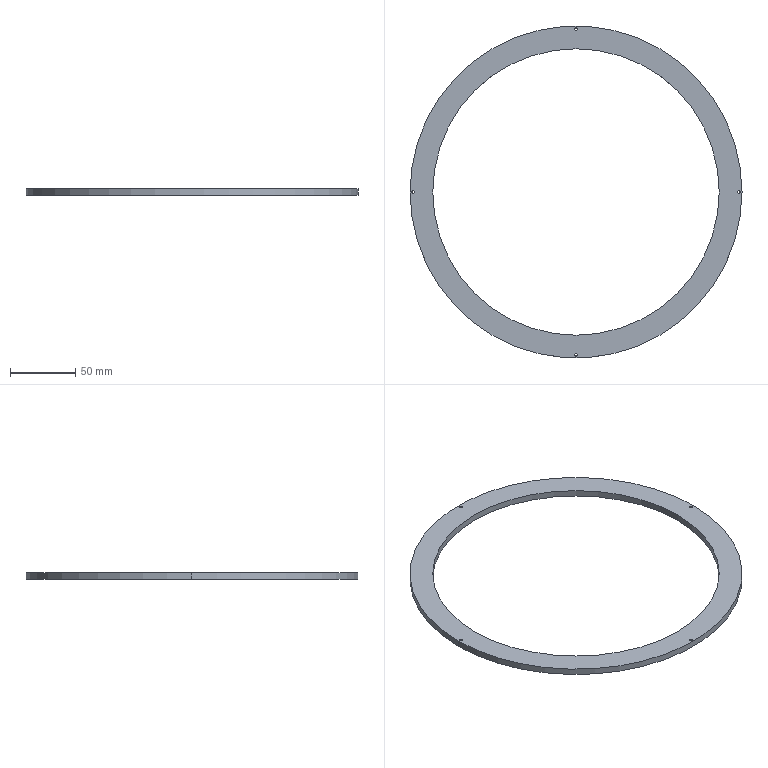Part | SolidWorks | features CirPattern 1, Extrusion 1, ICE 1 | 1 solid | 14 faces | box 255 x 255 x 5 mm | volume 65223 mm3 | cylinder 12 | plane 2 | commonest cylinder face diameters 2 x8 220 x2 255 x2
STEP:
#1=CARTESIAN_POINT('',(-126.,0.,0.));
#2=VERTEX_POINT('',#1);
#3=CARTESIAN_POINT('',(-124.,0.,0.));
#4=VERTEX_POINT('',#3);
#5=CARTESIAN_POINT('',(-125.,0.,0.));
#6=DIRECTION('',(0.,0.,1.));
#7=DIRECTION('',(0.,1.,0.));
#8=AXIS2_PLACEMENT_3D('',#5,#6,#7);
#9=CIRCLE('',#8,1.);
#10=EDGE_CURVE('',#2,#4,#9,.T.);
#11=ORIENTED_EDGE('',*,*,#10,.F.);
#12=CARTESIAN_POINT('',(-126.,0.,5.));
#13=VERTEX_POINT('',#12);
#14=CARTESIAN_POINT('',(-126.,0.,0.));
#15=DIRECTION('',(0.,0.,1.));
#16=VECTOR('',#15,1000.);
#17=LINE('',#14,#16);
#18=EDGE_CURVE('',#2,#13,#17,.T.);
#19=ORIENTED_EDGE('',*,*,#18,.T.);
#20=CARTESIAN_POINT('',(-124.,0.,5.));
#21=VERTEX_POINT('',#20);
#22=CARTESIAN_POINT('',(-125.,0.,5.));
#23=DIRECTION('',(0.,0.,1.));
#24=DIRECTION('',(0.,1.,0.));
#25=AXIS2_PLACEMENT_3D('',#22,#23,#24);
#26=CIRCLE('',#25,1.);
#27=EDGE_CURVE('',#13,#21,#26,.T.);
#28=ORIENTED_EDGE('',*,*,#27,.T.);
#29=CARTESIAN_POINT('',(-124.,0.,0.));
#30=DIRECTION('',(0.,0.,1.));
#31=VECTOR('',#30,1000.);
#32=LINE('',#29,#31);
#33=EDGE_CURVE('',#4,#21,#32,.T.);
#34=ORIENTED_EDGE('',*,*,#33,.F.);
#35=EDGE_LOOP('',(#11,#19,#28,#34));
#36=FACE_OUTER_BOUND('',#35,.T.);
#37=CARTESIAN_POINT('',(-125.,0.,0.));
#38=DIRECTION('',(0.,0.,1.));
#39=DIRECTION('',(1.,0.,0.));
#40=AXIS2_PLACEMENT_3D('',#37,#38,#39);
#41=CYLINDRICAL_SURFACE('',#40,1.);
#42=ADVANCED_FACE('',(#36),#41,.F.);
#43=CARTESIAN_POINT('',(-1.,-125.,0.));
#44=VERTEX_POINT('',#43);
#45=CARTESIAN_POINT('',(1.,-125.,0.));
#46=VERTEX_POINT('',#45);
#47=CARTESIAN_POINT('',(0.,-125.,0.));
#48=DIRECTION('',(0.,0.,1.));
#49=DIRECTION('',(-1.,0.,0.));
#50=AXIS2_PLACEMENT_3D('',#47,#48,#49);
#51=CIRCLE('',#50,1.);
#52=EDGE_CURVE('',#44,#46,#51,.T.);
#53=ORIENTED_EDGE('',*,*,#52,.F.);
#54=CARTESIAN_POINT('',(-1.,-125.,5.));
#55=VERTEX_POINT('',#54);
#56=CARTESIAN_POINT('',(-1.,-125.,0.));
#57=DIRECTION('',(0.,0.,1.));
#58=VECTOR('',#57,1000.);
#59=LINE('',#56,#58);
#60=EDGE_CURVE('',#44,#55,#59,.T.);
#61=ORIENTED_EDGE('',*,*,#60,.T.);
#62=CARTESIAN_POINT('',(1.,-125.,5.));
#63=VERTEX_POINT('',#62);
#64=CARTESIAN_POINT('',(0.,-125.,5.));
#65=DIRECTION('',(0.,0.,1.));
#66=DIRECTION('',(-1.,0.,0.));
#67=AXIS2_PLACEMENT_3D('',#64,#65,#66);
#68=CIRCLE('',#67,1.);
#69=EDGE_CURVE('',#55,#63,#68,.T.);
#70=ORIENTED_EDGE('',*,*,#69,.T.);
#71=CARTESIAN_POINT('',(1.,-125.,0.));
#72=DIRECTION('',(0.,0.,1.));
#73=VECTOR('',#72,1000.);
#74=LINE('',#71,#73);
#75=EDGE_CURVE('',#46,#63,#74,.T.);
#76=ORIENTED_EDGE('',*,*,#75,.F.);
#77=EDGE_LOOP('',(#53,#61,#70,#76));
#78=FACE_OUTER_BOUND('',#77,.T.);
#79=CARTESIAN_POINT('',(0.,-125.,0.));
#80=DIRECTION('',(0.,0.,1.));
#81=DIRECTION('',(1.,0.,0.));
#82=AXIS2_PLACEMENT_3D('',#79,#80,#81);
#83=CYLINDRICAL_SURFACE('',#82,1.);
#84=ADVANCED_FACE('',(#78),#83,.F.);
#85=CARTESIAN_POINT('',(124.,0.,0.));
#86=VERTEX_POINT('',#85);
#87=CARTESIAN_POINT('',(126.,0.,0.));
#88=VERTEX_POINT('',#87);
#89=CARTESIAN_POINT('',(125.,0.,0.));
#90=DIRECTION('',(0.,0.,1.));
#91=DIRECTION('',(0.,-1.,0.));
#92=AXIS2_PLACEMENT_3D('',#89,#90,#91);
#93=CIRCLE('',#92,1.);
#94=EDGE_CURVE('',#86,#88,#93,.T.);
#95=ORIENTED_EDGE('',*,*,#94,.F.);
#96=CARTESIAN_POINT('',(124.,0.,5.));
#97=VERTEX_POINT('',#96);
#98=CARTESIAN_POINT('',(124.,0.,0.));
#99=DIRECTION('',(0.,0.,1.));
#100=VECTOR('',#99,1000.);
#101=LINE('',#98,#100);
#102=EDGE_CURVE('',#86,#97,#101,.T.);
#103=ORIENTED_EDGE('',*,*,#102,.T.);
#104=CARTESIAN_POINT('',(126.,0.,5.));
#105=VERTEX_POINT('',#104);
#106=CARTESIAN_POINT('',(125.,0.,5.));
#107=DIRECTION('',(0.,0.,1.));
#108=DIRECTION('',(0.,-1.,0.));
#109=AXIS2_PLACEMENT_3D('',#106,#107,#108);
#110=CIRCLE('',#109,1.);
#111=EDGE_CURVE('',#97,#105,#110,.T.);
#112=ORIENTED_EDGE('',*,*,#111,.T.);
#113=CARTESIAN_POINT('',(126.,0.,0.));
#114=DIRECTION('',(0.,0.,1.));
#115=VECTOR('',#114,1000.);
#116=LINE('',#113,#115);
#117=EDGE_CURVE('',#88,#105,#116,.T.);
#118=ORIENTED_EDGE('',*,*,#117,.F.);
#119=EDGE_LOOP('',(#95,#103,#112,#118));
#120=FACE_OUTER_BOUND('',#119,.T.);
#121=CARTESIAN_POINT('',(125.,0.,0.));
#122=DIRECTION('',(0.,0.,1.));
#123=DIRECTION('',(1.,0.,0.));
#124=AXIS2_PLACEMENT_3D('',#121,#122,#123);
#125=CYLINDRICAL_SURFACE('',#124,1.);
#126=ADVANCED_FACE('',(#120),#125,.F.);
#127=CARTESIAN_POINT('',(-1.,125.,0.));
#128=VERTEX_POINT('',#127);
#129=CARTESIAN_POINT('',(1.,125.,0.));
#130=VERTEX_POINT('',#129);
#131=CARTESIAN_POINT('',(0.,125.,0.));
#132=DIRECTION('',(0.,0.,1.));
#133=DIRECTION('',(1.,0.,0.));
#134=AXIS2_PLACEMENT_3D('',#131,#132,#133);
#135=CIRCLE('',#134,1.);
#136=EDGE_CURVE('',#128,#130,#135,.T.);
#137=ORIENTED_EDGE('',*,*,#136,.F.);
#138=CARTESIAN_POINT('',(-1.,125.,5.));
#139=VERTEX_POINT('',#138);
#140=CARTESIAN_POINT('',(-1.,125.,0.));
#141=DIRECTION('',(0.,0.,1.));
#142=VECTOR('',#141,1000.);
#143=LINE('',#140,#142);
#144=EDGE_CURVE('',#128,#139,#143,.T.);
#145=ORIENTED_EDGE('',*,*,#144,.T.);
#146=CARTESIAN_POINT('',(1.,125.,5.));
#147=VERTEX_POINT('',#146);
#148=CARTESIAN_POINT('',(0.,125.,5.));
#149=DIRECTION('',(0.,0.,1.));
#150=DIRECTION('',(1.,0.,0.));
#151=AXIS2_PLACEMENT_3D('',#148,#149,#150);
#152=CIRCLE('',#151,1.);
#153=EDGE_CURVE('',#139,#147,#152,.T.);
#154=ORIENTED_EDGE('',*,*,#153,.T.);
#155=CARTESIAN_POINT('',(1.,125.,0.));
#156=DIRECTION('',(0.,0.,1.));
#157=VECTOR('',#156,1000.);
#158=LINE('',#155,#157);
#159=EDGE_CURVE('',#130,#147,#158,.T.);
#160=ORIENTED_EDGE('',*,*,#159,.F.);
#161=EDGE_LOOP('',(#137,#145,#154,#160));
#162=FACE_OUTER_BOUND('',#161,.T.);
#163=CARTESIAN_POINT('',(0.,125.,0.));
#164=DIRECTION('',(0.,0.,1.));
#165=DIRECTION('',(1.,0.,0.));
#166=AXIS2_PLACEMENT_3D('',#163,#164,#165);
#167=CYLINDRICAL_SURFACE('',#166,1.);
#168=ADVANCED_FACE('',(#162),#167,.F.);
#169=CARTESIAN_POINT('',(-110.,0.,5.));
#170=VERTEX_POINT('',#169);
#171=CARTESIAN_POINT('',(110.,0.,5.));
#172=VERTEX_POINT('',#171);
#173=CARTESIAN_POINT('',(0.,0.,5.));
#174=DIRECTION('',(0.,0.,1.));
#175=DIRECTION('',(1.,0.,0.));
#176=AXIS2_PLACEMENT_3D('',#173,#174,#175);
#177=CIRCLE('',#176,110.);
#178=EDGE_CURVE('',#170,#172,#177,.T.);
#179=ORIENTED_EDGE('',*,*,#178,.T.);
#180=CARTESIAN_POINT('',(110.,0.,0.));
#181=VERTEX_POINT('',#180);
#182=CARTESIAN_POINT('',(110.,0.,5.));
#183=DIRECTION('',(0.,0.,-1.));
#184=VECTOR('',#183,1000.);
#185=LINE('',#182,#184);
#186=EDGE_CURVE('',#172,#181,#185,.T.);
#187=ORIENTED_EDGE('',*,*,#186,.T.);
#188=CARTESIAN_POINT('',(-110.,0.,0.));
#189=VERTEX_POINT('',#188);
#190=CARTESIAN_POINT('',(0.,0.,0.));
#191=DIRECTION('',(0.,0.,1.));
#192=DIRECTION('',(1.,0.,0.));
#193=AXIS2_PLACEMENT_3D('',#190,#191,#192);
#194=CIRCLE('',#193,110.);
#195=EDGE_CURVE('',#189,#181,#194,.T.);
#196=ORIENTED_EDGE('',*,*,#195,.F.);
#197=CARTESIAN_POINT('',(-110.,0.,5.));
#198=DIRECTION('',(0.,0.,-1.));
#199=VECTOR('',#198,1000.);
#200=LINE('',#197,#199);
#201=EDGE_CURVE('',#170,#189,#200,.T.);
#202=ORIENTED_EDGE('',*,*,#201,.F.);
#203=EDGE_LOOP('',(#179,#187,#196,#202));
#204=FACE_OUTER_BOUND('',#203,.T.);
#205=CARTESIAN_POINT('',(0.,0.,5.));
#206=DIRECTION('',(0.,0.,-1.));
#207=DIRECTION('',(-1.,0.,0.));
#208=AXIS2_PLACEMENT_3D('',#205,#206,#207);
#209=CYLINDRICAL_SURFACE('',#208,110.);
#210=ADVANCED_FACE('',(#204),#209,.F.);
#211=CARTESIAN_POINT('',(127.5,0.,5.));
#212=VERTEX_POINT('',#211);
#213=CARTESIAN_POINT('',(-127.5,0.,5.));
#214=VERTEX_POINT('',#213);
#215=CARTESIAN_POINT('',(0.,0.,5.));
#216=DIRECTION('',(0.,0.,1.));
#217=DIRECTION('',(1.,0.,0.));
#218=AXIS2_PLACEMENT_3D('',#215,#216,#217);
#219=CIRCLE('',#218,127.5);
#220=EDGE_CURVE('',#212,#214,#219,.T.);
#221=ORIENTED_EDGE('',*,*,#220,.F.);
#222=CARTESIAN_POINT('',(127.5,0.,0.));
#223=VERTEX_POINT('',#222);
#224=CARTESIAN_POINT('',(127.5,0.,5.));
#225=DIRECTION('',(0.,0.,-1.));
#226=VECTOR('',#225,1000.);
#227=LINE('',#224,#226);
#228=EDGE_CURVE('',#212,#223,#227,.T.);
#229=ORIENTED_EDGE('',*,*,#228,.T.);
#230=CARTESIAN_POINT('',(-127.5,0.,0.));
#231=VERTEX_POINT('',#230);
#232=CARTESIAN_POINT('',(0.,0.,0.));
#233=DIRECTION('',(0.,0.,1.));
#234=DIRECTION('',(1.,0.,0.));
#235=AXIS2_PLACEMENT_3D('',#232,#233,#234);
#236=CIRCLE('',#235,127.5);
#237=EDGE_CURVE('',#223,#231,#236,.T.);
#238=ORIENTED_EDGE('',*,*,#237,.T.);
#239=CARTESIAN_POINT('',(-127.5,0.,5.));
#240=DIRECTION('',(0.,0.,-1.));
#241=VECTOR('',#240,1000.);
#242=LINE('',#239,#241);
#243=EDGE_CURVE('',#214,#231,#242,.T.);
#244=ORIENTED_EDGE('',*,*,#243,.F.);
#245=EDGE_LOOP('',(#221,#229,#238,#244));
#246=FACE_OUTER_BOUND('',#245,.T.);
#247=CARTESIAN_POINT('',(0.,0.,5.));
#248=DIRECTION('',(0.,0.,-1.));
#249=DIRECTION('',(-1.,0.,0.));
#250=AXIS2_PLACEMENT_3D('',#247,#248,#249);
#251=CYLINDRICAL_SURFACE('',#250,127.5);
#252=ADVANCED_FACE('',(#246),#251,.T.);
#253=CARTESIAN_POINT('',(-125.,0.,5.));
#254=DIRECTION('',(0.,0.,1.));
#255=DIRECTION('',(0.,1.,0.));
#256=AXIS2_PLACEMENT_3D('',#253,#254,#255);
#257=CIRCLE('',#256,1.);
#258=EDGE_CURVE('',#21,#13,#257,.T.);
#259=ORIENTED_EDGE('',*,*,#258,.F.);
#260=ORIENTED_EDGE('',*,*,#27,.F.);
#261=EDGE_LOOP('',(#259,#260));
#262=FACE_BOUND('',#261,.T.);
#263=CARTESIAN_POINT('',(0.,-125.,5.));
#264=DIRECTION('',(0.,0.,1.));
#265=DIRECTION('',(-1.,0.,0.));
#266=AXIS2_PLACEMENT_3D('',#263,#264,#265);
#267=CIRCLE('',#266,1.);
#268=EDGE_CURVE('',#63,#55,#267,.T.);
#269=ORIENTED_EDGE('',*,*,#268,.F.);
#270=ORIENTED_EDGE('',*,*,#69,.F.);
#271=EDGE_LOOP('',(#269,#270));
#272=FACE_BOUND('',#271,.T.);
#273=CARTESIAN_POINT('',(125.,0.,5.));
#274=DIRECTION('',(0.,0.,1.));
#275=DIRECTION('',(0.,-1.,0.));
#276=AXIS2_PLACEMENT_3D('',#273,#274,#275);
#277=CIRCLE('',#276,1.);
#278=EDGE_CURVE('',#105,#97,#277,.T.);
#279=ORIENTED_EDGE('',*,*,#278,.F.);
#280=ORIENTED_EDGE('',*,*,#111,.F.);
#281=EDGE_LOOP('',(#279,#280));
#282=FACE_BOUND('',#281,.T.);
#283=CARTESIAN_POINT('',(0.,125.,5.));
#284=DIRECTION('',(0.,0.,1.));
#285=DIRECTION('',(1.,0.,0.));
#286=AXIS2_PLACEMENT_3D('',#283,#284,#285);
#287=CIRCLE('',#286,1.);
#288=EDGE_CURVE('',#147,#139,#287,.T.);
#289=ORIENTED_EDGE('',*,*,#288,.F.);
#290=ORIENTED_EDGE('',*,*,#153,.F.);
#291=EDGE_LOOP('',(#289,#290));
#292=FACE_BOUND('',#291,.T.);
#293=CARTESIAN_POINT('',(0.,0.,5.));
#294=DIRECTION('',(0.,0.,1.));
#295=DIRECTION('',(1.,0.,0.));
#296=AXIS2_PLACEMENT_3D('',#293,#294,#295);
#297=CIRCLE('',#296,127.5);
#298=EDGE_CURVE('',#214,#212,#297,.T.);
#299=ORIENTED_EDGE('',*,*,#298,.T.);
#300=ORIENTED_EDGE('',*,*,#220,.T.);
#301=EDGE_LOOP('',(#299,#300));
#302=FACE_OUTER_BOUND('',#301,.T.);
#303=ORIENTED_EDGE('',*,*,#178,.F.);
#304=CARTESIAN_POINT('',(0.,0.,5.));
#305=DIRECTION('',(0.,0.,1.));
#306=DIRECTION('',(1.,0.,0.));
#307=AXIS2_PLACEMENT_3D('',#304,#305,#306);
#308=CIRCLE('',#307,110.);
#309=EDGE_CURVE('',#172,#170,#308,.T.);
#310=ORIENTED_EDGE('',*,*,#309,.F.);
#311=EDGE_LOOP('',(#303,#310));
#312=FACE_BOUND('',#311,.T.);
#313=CARTESIAN_POINT('',(0.,0.,5.));
#314=DIRECTION('',(0.,0.,1.));
#315=DIRECTION('',(1.,0.,0.));
#316=AXIS2_PLACEMENT_3D('',#313,#314,#315);
#317=PLANE('',#316);
#318=ADVANCED_FACE('',(#262,#272,#282,#292,#302,#312),#317,.T.);
#319=CARTESIAN_POINT('',(-125.,0.,0.));
#320=DIRECTION('',(0.,0.,1.));
#321=DIRECTION('',(0.,1.,0.));
#322=AXIS2_PLACEMENT_3D('',#319,#320,#321);
#323=CIRCLE('',#322,1.);
#324=EDGE_CURVE('',#4,#2,#323,.T.);
#325=ORIENTED_EDGE('',*,*,#324,.T.);
#326=ORIENTED_EDGE('',*,*,#10,.T.);
#327=EDGE_LOOP('',(#325,#326));
#328=FACE_BOUND('',#327,.T.);
#329=CARTESIAN_POINT('',(0.,-125.,0.));
#330=DIRECTION('',(0.,0.,1.));
#331=DIRECTION('',(-1.,0.,0.));
#332=AXIS2_PLACEMENT_3D('',#329,#330,#331);
#333=CIRCLE('',#332,1.);
#334=EDGE_CURVE('',#46,#44,#333,.T.);
#335=ORIENTED_EDGE('',*,*,#334,.T.);
#336=ORIENTED_EDGE('',*,*,#52,.T.);
#337=EDGE_LOOP('',(#335,#336));
#338=FACE_BOUND('',#337,.T.);
#339=CARTESIAN_POINT('',(125.,0.,0.));
#340=DIRECTION('',(0.,0.,1.));
#341=DIRECTION('',(0.,-1.,0.));
#342=AXIS2_PLACEMENT_3D('',#339,#340,#341);
#343=CIRCLE('',#342,1.);
#344=EDGE_CURVE('',#88,#86,#343,.T.);
#345=ORIENTED_EDGE('',*,*,#344,.T.);
#346=ORIENTED_EDGE('',*,*,#94,.T.);
#347=EDGE_LOOP('',(#345,#346));
#348=FACE_BOUND('',#347,.T.);
#349=CARTESIAN_POINT('',(0.,125.,0.));
#350=DIRECTION('',(0.,0.,1.));
#351=DIRECTION('',(1.,0.,0.));
#352=AXIS2_PLACEMENT_3D('',#349,#350,#351);
#353=CIRCLE('',#352,1.);
#354=EDGE_CURVE('',#130,#128,#353,.T.);
#355=ORIENTED_EDGE('',*,*,#354,.T.);
#356=ORIENTED_EDGE('',*,*,#136,.T.);
#357=EDGE_LOOP('',(#355,#356));
#358=FACE_BOUND('',#357,.T.);
#359=CARTESIAN_POINT('',(0.,0.,0.));
#360=DIRECTION('',(0.,0.,1.));
#361=DIRECTION('',(1.,0.,0.));
#362=AXIS2_PLACEMENT_3D('',#359,#360,#361);
#363=CIRCLE('',#362,127.5);
#364=EDGE_CURVE('',#231,#223,#363,.T.);
#365=ORIENTED_EDGE('',*,*,#364,.F.);
#366=ORIENTED_EDGE('',*,*,#237,.F.);
#367=EDGE_LOOP('',(#365,#366));
#368=FACE_OUTER_BOUND('',#367,.T.);
#369=ORIENTED_EDGE('',*,*,#195,.T.);
#370=CARTESIAN_POINT('',(0.,0.,0.));
#371=DIRECTION('',(0.,0.,1.));
#372=DIRECTION('',(1.,0.,0.));
#373=AXIS2_PLACEMENT_3D('',#370,#371,#372);
#374=CIRCLE('',#373,110.);
#375=EDGE_CURVE('',#181,#189,#374,.T.);
#376=ORIENTED_EDGE('',*,*,#375,.T.);
#377=EDGE_LOOP('',(#369,#376));
#378=FACE_BOUND('',#377,.T.);
#379=CARTESIAN_POINT('',(0.,0.,0.));
#380=DIRECTION('',(0.,0.,1.));
#381=DIRECTION('',(1.,0.,0.));
#382=AXIS2_PLACEMENT_3D('',#379,#380,#381);
#383=PLANE('',#382);
#384=ADVANCED_FACE('',(#328,#338,#348,#358,#368,#378),#383,.F.);
#385=ORIENTED_EDGE('',*,*,#228,.F.);
#386=ORIENTED_EDGE('',*,*,#298,.F.);
#387=ORIENTED_EDGE('',*,*,#243,.T.);
#388=ORIENTED_EDGE('',*,*,#364,.T.);
#389=EDGE_LOOP('',(#385,#386,#387,#388));
#390=FACE_OUTER_BOUND('',#389,.T.);
#391=CARTESIAN_POINT('',(0.,0.,5.));
#392=DIRECTION('',(0.,0.,-1.));
#393=DIRECTION('',(-1.,0.,0.));
#394=AXIS2_PLACEMENT_3D('',#391,#392,#393);
#395=CYLINDRICAL_SURFACE('',#394,127.5);
#396=ADVANCED_FACE('',(#390),#395,.T.);
#397=ORIENTED_EDGE('',*,*,#186,.F.);
#398=ORIENTED_EDGE('',*,*,#309,.T.);
#399=ORIENTED_EDGE('',*,*,#201,.T.);
#400=ORIENTED_EDGE('',*,*,#375,.F.);
#401=EDGE_LOOP('',(#397,#398,#399,#400));
#402=FACE_OUTER_BOUND('',#401,.T.);
#403=CARTESIAN_POINT('',(0.,0.,5.));
#404=DIRECTION('',(0.,0.,-1.));
#405=DIRECTION('',(-1.,0.,0.));
#406=AXIS2_PLACEMENT_3D('',#403,#404,#405);
#407=CYLINDRICAL_SURFACE('',#406,110.);
#408=ADVANCED_FACE('',(#402),#407,.F.);
#409=ORIENTED_EDGE('',*,*,#144,.F.);
#410=ORIENTED_EDGE('',*,*,#354,.F.);
#411=ORIENTED_EDGE('',*,*,#159,.T.);
#412=ORIENTED_EDGE('',*,*,#288,.T.);
#413=EDGE_LOOP('',(#409,#410,#411,#412));
#414=FACE_OUTER_BOUND('',#413,.T.);
#415=CARTESIAN_POINT('',(0.,125.,0.));
#416=DIRECTION('',(0.,0.,1.));
#417=DIRECTION('',(1.,0.,0.));
#418=AXIS2_PLACEMENT_3D('',#415,#416,#417);
#419=CYLINDRICAL_SURFACE('',#418,1.);
#420=ADVANCED_FACE('',(#414),#419,.F.);
#421=ORIENTED_EDGE('',*,*,#102,.F.);
#422=ORIENTED_EDGE('',*,*,#344,.F.);
#423=ORIENTED_EDGE('',*,*,#117,.T.);
#424=ORIENTED_EDGE('',*,*,#278,.T.);
#425=EDGE_LOOP('',(#421,#422,#423,#424));
#426=FACE_OUTER_BOUND('',#425,.T.);
#427=CARTESIAN_POINT('',(125.,0.,0.));
#428=DIRECTION('',(0.,0.,1.));
#429=DIRECTION('',(1.,0.,0.));
#430=AXIS2_PLACEMENT_3D('',#427,#428,#429);
#431=CYLINDRICAL_SURFACE('',#430,1.);
#432=ADVANCED_FACE('',(#426),#431,.F.);
#433=ORIENTED_EDGE('',*,*,#60,.F.);
#434=ORIENTED_EDGE('',*,*,#334,.F.);
#435=ORIENTED_EDGE('',*,*,#75,.T.);
#436=ORIENTED_EDGE('',*,*,#268,.T.);
#437=EDGE_LOOP('',(#433,#434,#435,#436));
#438=FACE_OUTER_BOUND('',#437,.T.);
#439=CARTESIAN_POINT('',(0.,-125.,0.));
#440=DIRECTION('',(0.,0.,1.));
#441=DIRECTION('',(1.,0.,0.));
#442=AXIS2_PLACEMENT_3D('',#439,#440,#441);
#443=CYLINDRICAL_SURFACE('',#442,1.);
#444=ADVANCED_FACE('',(#438),#443,.F.);
#445=ORIENTED_EDGE('',*,*,#18,.F.);
#446=ORIENTED_EDGE('',*,*,#324,.F.);
#447=ORIENTED_EDGE('',*,*,#33,.T.);
#448=ORIENTED_EDGE('',*,*,#258,.T.);
#449=EDGE_LOOP('',(#445,#446,#447,#448));
#450=FACE_OUTER_BOUND('',#449,.T.);
#451=CARTESIAN_POINT('',(-125.,0.,0.));
#452=DIRECTION('',(0.,0.,1.));
#453=DIRECTION('',(1.,0.,0.));
#454=AXIS2_PLACEMENT_3D('',#451,#452,#453);
#455=CYLINDRICAL_SURFACE('',#454,1.);
#456=ADVANCED_FACE('',(#450),#455,.F.);
#457=CLOSED_SHELL('',(#42,#84,#126,#168,#210,#252,#318,#384,#396,#408,#420,#432,#444,#456));
#458=MANIFOLD_SOLID_BREP('',#457);
#459=CARTESIAN_POINT('',(0.,0.,0.));
#460=DIRECTION('',(0.,0.,1.));
#461=DIRECTION('',(1.,0.,0.));
#462=AXIS2_PLACEMENT_3D('',#459,#460,#461);
#463=(LENGTH_UNIT()NAMED_UNIT(*)SI_UNIT(.MILLI.,.METRE.));
#464=UNCERTAINTY_MEASURE_WITH_UNIT(LENGTH_MEASURE(0.00001),#463,'','');
#465=(NAMED_UNIT(*)PLANE_ANGLE_UNIT()SI_UNIT($,.RADIAN.));
#466=(NAMED_UNIT(*)SI_UNIT($,.STERADIAN.)SOLID_ANGLE_UNIT());
#467=(GEOMETRIC_REPRESENTATION_CONTEXT(3)GLOBAL_UNCERTAINTY_ASSIGNED_CONTEXT((#464))GLOBAL_UNIT_ASSIGNED_CONTEXT((#463,#465,#466))REPRESENTATION_CONTEXT('',''));
#468=ADVANCED_BREP_SHAPE_REPRESENTATION('',(#458,#462),#467);